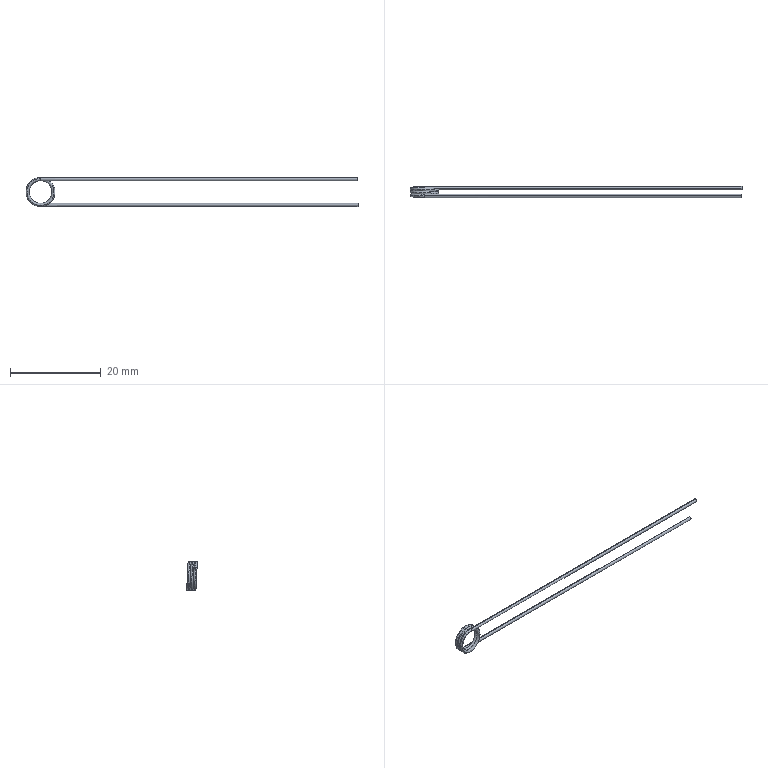Part | SolidWorks | features MoveFace 2, CompositeCurve 1, Helix 1, Sweep 1 | 1 solid | 9 faces | box 73.25 x 2.45 x 6.4 mm | volume 70.525 mm3 | cylinder 4 | spline 3 | plane 2 | commonest cylinder face diameters 0.7 x4
STEP:
#1=CARTESIAN_POINT('',(70.05,1.75,-3.2));
#2=VERTEX_POINT('',#1);
#3=CARTESIAN_POINT('',(70.05,1.75,-2.5));
#4=VERTEX_POINT('',#3);
#5=CARTESIAN_POINT('',(70.05,1.75,-2.85));
#6=DIRECTION('',(1.,0.,0.));
#7=DIRECTION('',(0.,0.00009155,-1.));
#8=AXIS2_PLACEMENT_3D('',#5,#6,#7);
#9=CIRCLE('',#8,0.35);
#10=EDGE_CURVE('',#2,#4,#9,.T.);
#11=ORIENTED_EDGE('',*,*,#10,.F.);
#12=CARTESIAN_POINT('',(-0.000000536,1.75,-3.2));
#13=VERTEX_POINT('',#12);
#14=CARTESIAN_POINT('',(12.85,1.75,-3.2));
#15=DIRECTION('',(-1.,0.,0.));
#16=VECTOR('',#15,1000.);
#17=LINE('',#14,#16);
#18=EDGE_CURVE('',#2,#13,#17,.T.);
#19=ORIENTED_EDGE('',*,*,#18,.T.);
#20=CARTESIAN_POINT('',(-0.006305,2.074,-2.979));
#21=VERTEX_POINT('',#20);
#22=CARTESIAN_POINT('',(0.,1.75,-2.85));
#23=DIRECTION('',(1.,0.,0.));
#24=DIRECTION('',(0.,0.00009155,-1.));
#25=AXIS2_PLACEMENT_3D('',#22,#23,#24);
#26=CIRCLE('',#25,0.35);
#27=EDGE_CURVE('',#13,#21,#26,.T.);
#28=ORIENTED_EDGE('',*,*,#27,.T.);
#29=CARTESIAN_POINT('',(0.,1.75,-2.5));
#30=VERTEX_POINT('',#29);
#31=CARTESIAN_POINT('',(0.,1.75,-2.85));
#32=DIRECTION('',(1.,0.,0.));
#33=DIRECTION('',(0.,0.00009155,-1.));
#34=AXIS2_PLACEMENT_3D('',#31,#32,#33);
#35=CIRCLE('',#34,0.35);
#36=EDGE_CURVE('',#21,#30,#35,.T.);
#37=ORIENTED_EDGE('',*,*,#36,.T.);
#38=CARTESIAN_POINT('',(12.85,1.75,-2.5));
#39=DIRECTION('',(-1.,0.,0.));
#40=VECTOR('',#39,1000.);
#41=LINE('',#38,#40);
#42=EDGE_CURVE('',#4,#30,#41,.T.);
#43=ORIENTED_EDGE('',*,*,#42,.F.);
#44=EDGE_LOOP('',(#11,#19,#28,#37,#43));
#45=FACE_OUTER_BOUND('',#44,.T.);
#46=CARTESIAN_POINT('',(12.85,1.75,-2.85));
#47=DIRECTION('',(-1.,0.,0.));
#48=DIRECTION('',(0.,0.,1.));
#49=AXIS2_PLACEMENT_3D('',#46,#47,#48);
#50=CYLINDRICAL_SURFACE('',#49,0.35);
#51=ADVANCED_FACE('',(#45),#50,.T.);
#52=CARTESIAN_POINT('',(0.006305,0.3239,2.979));
#53=VERTEX_POINT('',#52);
#54=CARTESIAN_POINT('',(0.,0.,3.2));
#55=VERTEX_POINT('',#54);
#56=CARTESIAN_POINT('',(0.006305,0.3239,2.979));
#57=CARTESIAN_POINT('',(0.01048,0.2681,3.104));
#58=CARTESIAN_POINT('',(0.005425,0.1388,3.2));
#59=CARTESIAN_POINT('',(0.,0.,3.2));
#60=B_SPLINE_CURVE_WITH_KNOTS('',3,(#56,#57,#58,#59),.UNSPECIFIED.,.F.,.F.,(4,4),(0.00002721,0.1895),.UNSPECIFIED.);
#61=EDGE_CURVE('',#53,#55,#60,.T.);
#62=ORIENTED_EDGE('',*,*,#61,.T.);
#63=CARTESIAN_POINT('',(70.05,0.,3.2));
#64=VERTEX_POINT('',#63);
#65=CARTESIAN_POINT('',(0.,0.,3.2));
#66=DIRECTION('',(1.,0.,0.));
#67=VECTOR('',#66,1000.);
#68=LINE('',#65,#67);
#69=EDGE_CURVE('',#55,#64,#68,.T.);
#70=ORIENTED_EDGE('',*,*,#69,.T.);
#71=CARTESIAN_POINT('',(70.05,0.,2.5));
#72=VERTEX_POINT('',#71);
#73=CARTESIAN_POINT('',(70.05,0.,2.85));
#74=DIRECTION('',(-1.,0.,0.));
#75=DIRECTION('',(0.,0.,1.));
#76=AXIS2_PLACEMENT_3D('',#73,#74,#75);
#77=CIRCLE('',#76,0.35);
#78=EDGE_CURVE('',#64,#72,#77,.T.);
#79=ORIENTED_EDGE('',*,*,#78,.T.);
#80=CARTESIAN_POINT('',(0.,0.,2.5));
#81=VERTEX_POINT('',#80);
#82=CARTESIAN_POINT('',(0.,0.,2.5));
#83=DIRECTION('',(1.,0.,0.));
#84=VECTOR('',#83,1000.);
#85=LINE('',#82,#84);
#86=EDGE_CURVE('',#81,#72,#85,.T.);
#87=ORIENTED_EDGE('',*,*,#86,.F.);
#88=CARTESIAN_POINT('',(0.,0.,2.85));
#89=DIRECTION('',(-1.,0.,0.));
#90=DIRECTION('',(0.,0.,1.));
#91=AXIS2_PLACEMENT_3D('',#88,#89,#90);
#92=CIRCLE('',#91,0.35);
#93=EDGE_CURVE('',#53,#81,#92,.T.);
#94=ORIENTED_EDGE('',*,*,#93,.F.);
#95=EDGE_LOOP('',(#62,#70,#79,#87,#94));
#96=FACE_OUTER_BOUND('',#95,.T.);
#97=CARTESIAN_POINT('',(0.,0.,2.85));
#98=DIRECTION('',(1.,0.,0.));
#99=DIRECTION('',(0.,0.,-1.));
#100=AXIS2_PLACEMENT_3D('',#97,#98,#99);
#101=CYLINDRICAL_SURFACE('',#100,0.35);
#102=ADVANCED_FACE('',(#96),#101,.T.);
#103=ORIENTED_EDGE('',*,*,#18,.F.);
#104=CARTESIAN_POINT('',(70.05,1.75,-2.85));
#105=DIRECTION('',(1.,0.,0.));
#106=DIRECTION('',(0.,0.00009155,-1.));
#107=AXIS2_PLACEMENT_3D('',#104,#105,#106);
#108=CIRCLE('',#107,0.35);
#109=EDGE_CURVE('',#4,#2,#108,.T.);
#110=ORIENTED_EDGE('',*,*,#109,.F.);
#111=ORIENTED_EDGE('',*,*,#42,.T.);
#112=CARTESIAN_POINT('',(0.006304,1.426,-2.979));
#113=VERTEX_POINT('',#112);
#114=CARTESIAN_POINT('',(0.,1.75,-2.85));
#115=DIRECTION('',(1.,0.,0.));
#116=DIRECTION('',(0.,0.00009155,-1.));
#117=AXIS2_PLACEMENT_3D('',#114,#115,#116);
#118=CIRCLE('',#117,0.35);
#119=EDGE_CURVE('',#30,#113,#118,.T.);
#120=ORIENTED_EDGE('',*,*,#119,.T.);
#121=CARTESIAN_POINT('',(0.,1.75,-2.85));
#122=DIRECTION('',(1.,0.,0.));
#123=DIRECTION('',(0.,0.00009155,-1.));
#124=AXIS2_PLACEMENT_3D('',#121,#122,#123);
#125=CIRCLE('',#124,0.35);
#126=EDGE_CURVE('',#113,#13,#125,.T.);
#127=ORIENTED_EDGE('',*,*,#126,.T.);
#128=EDGE_LOOP('',(#103,#110,#111,#120,#127));
#129=FACE_OUTER_BOUND('',#128,.T.);
#130=CARTESIAN_POINT('',(12.85,1.75,-2.85));
#131=DIRECTION('',(-1.,0.,0.));
#132=DIRECTION('',(0.,0.,1.));
#133=AXIS2_PLACEMENT_3D('',#130,#131,#132);
#134=CYLINDRICAL_SURFACE('',#133,0.35);
#135=ADVANCED_FACE('',(#129),#134,.T.);
#136=ORIENTED_EDGE('',*,*,#36,.F.);
#137=CARTESIAN_POINT('',(0.006305,0.3239,2.979));
#138=CARTESIAN_POINT('',(-0.7712,0.3519,2.981));
#139=CARTESIAN_POINT('',(-1.545,0.381,2.663));
#140=CARTESIAN_POINT('',(-2.649,0.4392,1.566));
#141=CARTESIAN_POINT('',(-2.975,0.4683,0.7939));
#142=CARTESIAN_POINT('',(-2.98,0.5195,-0.5733));
#143=CARTESIAN_POINT('',(-2.806,0.5413,-1.156));
#144=CARTESIAN_POINT('',(-2.162,0.585,-2.13));
#145=CARTESIAN_POINT('',(-1.69,0.6069,-2.521));
#146=CARTESIAN_POINT('',(-0.4324,0.658,-3.048));
#147=CARTESIAN_POINT('',(0.405,0.6871,-3.052));
#148=CARTESIAN_POINT('',(1.67,0.7383,-2.534));
#149=CARTESIAN_POINT('',(2.142,0.7601,-2.15));
#150=CARTESIAN_POINT('',(2.795,0.8037,-1.182));
#151=CARTESIAN_POINT('',(2.976,0.8257,-0.5972));
#152=CARTESIAN_POINT('',(2.981,0.8768,0.7668));
#153=CARTESIAN_POINT('',(2.665,0.9058,1.542));
#154=CARTESIAN_POINT('',(1.702,0.957,2.513));
#155=CARTESIAN_POINT('',(1.167,0.9788,2.801));
#156=CARTESIAN_POINT('',(0.02248,1.022,3.035));
#157=CARTESIAN_POINT('',(-0.587,1.044,2.978));
#158=CARTESIAN_POINT('',(-1.849,1.096,2.461));
#159=CARTESIAN_POINT('',(-2.445,1.125,1.872));
#160=CARTESIAN_POINT('',(-2.973,1.176,0.6109));
#161=CARTESIAN_POINT('',(-3.035,1.198,0.005944));
#162=CARTESIAN_POINT('',(-2.812,1.241,-1.14));
#163=CARTESIAN_POINT('',(-2.526,1.263,-1.682));
#164=CARTESIAN_POINT('',(-1.566,1.314,-2.65));
#165=CARTESIAN_POINT('',(-0.7938,1.343,-2.975));
#166=CARTESIAN_POINT('',(0.5733,1.395,-2.98));
#167=CARTESIAN_POINT('',(1.156,1.416,-2.806));
#168=CARTESIAN_POINT('',(2.13,1.46,-2.162));
#169=CARTESIAN_POINT('',(2.521,1.482,-1.69));
#170=CARTESIAN_POINT('',(3.048,1.533,-0.4324));
#171=CARTESIAN_POINT('',(3.052,1.562,0.405));
#172=CARTESIAN_POINT('',(2.534,1.613,1.67));
#173=CARTESIAN_POINT('',(2.15,1.635,2.142));
#174=CARTESIAN_POINT('',(1.182,1.679,2.795));
#175=CARTESIAN_POINT('',(0.5972,1.701,2.976));
#176=CARTESIAN_POINT('',(-0.7668,1.752,2.981));
#177=CARTESIAN_POINT('',(-1.542,1.781,2.665));
#178=CARTESIAN_POINT('',(-2.513,1.832,1.702));
#179=CARTESIAN_POINT('',(-2.801,1.854,1.167));
#180=CARTESIAN_POINT('',(-3.034,1.897,0.0225));
#181=CARTESIAN_POINT('',(-2.978,1.919,-0.587));
#182=CARTESIAN_POINT('',(-2.46,1.971,-1.85));
#183=CARTESIAN_POINT('',(-1.872,2.,-2.445));
#184=CARTESIAN_POINT('',(-0.7917,2.043,-2.897));
#185=CARTESIAN_POINT('',(-0.4042,2.058,-2.976));
#186=CARTESIAN_POINT('',(-0.006305,2.074,-2.979));
#187=B_SPLINE_CURVE_WITH_KNOTS('',3,(#137,#138,#139,#140,#141,#142,#143,#144,#145,#146,#147,#148,#149,#150,#151,#152,#153,#154,#155,#156,#157,#158,#159,#160,#161,#162,#163,#164,#165,#166,#167,#168,#169,#170,#171,#172,#173,#174,#175,#176,#177,#178,#179,#180,#181,#182,#183,#184,#185,#186),.UNSPECIFIED.,.F.,.F.,(4,2,2,2,2,2,2,2,2,2,2,2,2,2,2,2,2,2,2,2,2,2,2,2,4),(0.,0.04998,0.09999,0.1375,0.175,0.225,0.2625,0.3,0.35,0.3875,0.425,0.475,0.5125,0.55,0.6,0.6375,0.675,0.725,0.7625,0.8,0.85,0.8875,0.925,0.975,1.),.UNSPECIFIED.);
#188=EDGE_CURVE('',#53,#21,#187,.T.);
#189=ORIENTED_EDGE('',*,*,#188,.F.);
#190=ORIENTED_EDGE('',*,*,#93,.T.);
#191=CARTESIAN_POINT('',(-0.006304,-0.3239,2.979));
#192=VERTEX_POINT('',#191);
#193=CARTESIAN_POINT('',(0.,0.,2.85));
#194=DIRECTION('',(-1.,0.,0.));
#195=DIRECTION('',(0.,0.,1.));
#196=AXIS2_PLACEMENT_3D('',#193,#194,#195);
#197=CIRCLE('',#196,0.35);
#198=EDGE_CURVE('',#81,#192,#197,.T.);
#199=ORIENTED_EDGE('',*,*,#198,.T.);
#200=CARTESIAN_POINT('',(0.006304,1.426,-2.979));
#201=CARTESIAN_POINT('',(-0.379,1.413,-2.98));
#202=CARTESIAN_POINT('',(-0.7673,1.398,-2.904));
#203=CARTESIAN_POINT('',(-1.851,1.354,-2.461));
#204=CARTESIAN_POINT('',(-2.445,1.325,-1.871));
#205=CARTESIAN_POINT('',(-2.973,1.274,-0.6122));
#206=CARTESIAN_POINT('',(-3.035,1.252,-0.003211));
#207=CARTESIAN_POINT('',(-2.811,1.209,1.143));
#208=CARTESIAN_POINT('',(-2.527,1.187,1.681));
#209=CARTESIAN_POINT('',(-1.565,1.136,2.652));
#210=CARTESIAN_POINT('',(-0.792,1.107,2.975));
#211=CARTESIAN_POINT('',(0.572,1.056,2.981));
#212=CARTESIAN_POINT('',(1.158,1.034,2.805));
#213=CARTESIAN_POINT('',(2.132,0.99,2.16));
#214=CARTESIAN_POINT('',(2.52,0.9682,1.692));
#215=CARTESIAN_POINT('',(3.049,0.917,0.4308));
#216=CARTESIAN_POINT('',(3.052,0.8879,-0.4067));
#217=CARTESIAN_POINT('',(2.535,0.8368,-1.669));
#218=CARTESIAN_POINT('',(2.148,0.8149,-2.144));
#219=CARTESIAN_POINT('',(1.18,0.7712,-2.796));
#220=CARTESIAN_POINT('',(0.5985,0.7494,-2.976));
#221=CARTESIAN_POINT('',(-0.7686,0.6982,-2.981));
#222=CARTESIAN_POINT('',(-1.544,0.6692,-2.664));
#223=CARTESIAN_POINT('',(-2.512,0.6181,-1.703));
#224=CARTESIAN_POINT('',(-2.802,0.5961,-1.164));
#225=CARTESIAN_POINT('',(-3.035,0.5525,-0.01977));
#226=CARTESIAN_POINT('',(-2.978,0.5307,0.5858));
#227=CARTESIAN_POINT('',(-2.46,0.4795,1.851));
#228=CARTESIAN_POINT('',(-1.87,0.4504,2.445));
#229=CARTESIAN_POINT('',(-0.6122,0.3993,2.973));
#230=CARTESIAN_POINT('',(-0.003226,0.3774,3.035));
#231=CARTESIAN_POINT('',(1.143,0.3337,2.811));
#232=CARTESIAN_POINT('',(1.681,0.3119,2.527));
#233=CARTESIAN_POINT('',(2.652,0.2607,1.565));
#234=CARTESIAN_POINT('',(2.975,0.2317,0.792));
#235=CARTESIAN_POINT('',(2.981,0.1806,-0.572));
#236=CARTESIAN_POINT('',(2.805,0.1586,-1.158));
#237=CARTESIAN_POINT('',(2.16,0.115,-2.132));
#238=CARTESIAN_POINT('',(1.692,0.09317,-2.52));
#239=CARTESIAN_POINT('',(0.4308,0.04196,-3.049));
#240=CARTESIAN_POINT('',(-0.4067,0.01292,-3.052));
#241=CARTESIAN_POINT('',(-1.669,-0.03818,-2.535));
#242=CARTESIAN_POINT('',(-2.144,-0.06013,-2.148));
#243=CARTESIAN_POINT('',(-2.796,-0.1038,-1.18));
#244=CARTESIAN_POINT('',(-2.976,-0.1256,-0.5985));
#245=CARTESIAN_POINT('',(-2.981,-0.1768,0.7687));
#246=CARTESIAN_POINT('',(-2.663,-0.2059,1.544));
#247=CARTESIAN_POINT('',(-1.567,-0.2642,2.65));
#248=CARTESIAN_POINT('',(-0.7966,-0.2932,2.975));
#249=CARTESIAN_POINT('',(-0.006304,-0.3239,2.979));
#250=B_SPLINE_CURVE_WITH_KNOTS('',3,(#200,#201,#202,#203,#204,#205,#206,#207,#208,#209,#210,#211,#212,#213,#214,#215,#216,#217,#218,#219,#220,#221,#222,#223,#224,#225,#226,#227,#228,#229,#230,#231,#232,#233,#234,#235,#236,#237,#238,#239,#240,#241,#242,#243,#244,#245,#246,#247,#248,#249),.UNSPECIFIED.,.F.,.F.,(4,2,2,2,2,2,2,2,2,2,2,2,2,2,2,2,2,2,2,2,2,2,2,2,4),(0.,0.02496,0.07501,0.1125,0.15,0.2,0.2375,0.275,0.325,0.3625,0.4,0.45,0.4875,0.525,0.575,0.6125,0.65,0.7,0.7375,0.775,0.825,0.8625,0.9,0.95,1.),.UNSPECIFIED.);
#251=EDGE_CURVE('',#113,#192,#250,.T.);
#252=ORIENTED_EDGE('',*,*,#251,.F.);
#253=ORIENTED_EDGE('',*,*,#119,.F.);
#254=EDGE_LOOP('',(#136,#189,#190,#199,#252,#253));
#255=FACE_OUTER_BOUND('',#254,.T.);
#256=CARTESIAN_POINT('',(-0.01261,2.073,-2.978));
#257=CARTESIAN_POINT('',(-0.9931,2.036,-2.974));
#258=CARTESIAN_POINT('',(-1.942,2.,-2.452));
#259=CARTESIAN_POINT('',(-3.022,1.927,-0.8338));
#260=CARTESIAN_POINT('',(-3.123,1.89,0.2539));
#261=CARTESIAN_POINT('',(-2.369,1.817,2.048));
#262=CARTESIAN_POINT('',(-1.523,1.781,2.732));
#263=CARTESIAN_POINT('',(0.3864,1.708,3.111));
#264=CARTESIAN_POINT('',(1.43,1.671,2.788));
#265=CARTESIAN_POINT('',(2.798,1.599,1.405));
#266=CARTESIAN_POINT('',(3.107,1.562,0.3615));
#267=CARTESIAN_POINT('',(2.726,1.489,-1.547));
#268=CARTESIAN_POINT('',(2.029,1.453,-2.388));
#269=CARTESIAN_POINT('',(0.2273,1.38,-3.123));
#270=CARTESIAN_POINT('',(-0.8551,1.343,-3.009));
#271=CARTESIAN_POINT('',(-2.473,1.271,-1.927));
#272=CARTESIAN_POINT('',(-2.982,1.234,-0.9604));
#273=CARTESIAN_POINT('',(-2.972,1.161,0.9852));
#274=CARTESIAN_POINT('',(-2.453,1.125,1.942));
#275=CARTESIAN_POINT('',(-0.8335,1.052,3.022));
#276=CARTESIAN_POINT('',(0.2539,1.015,3.123));
#277=CARTESIAN_POINT('',(2.048,0.9425,2.369));
#278=CARTESIAN_POINT('',(2.732,0.9059,1.523));
#279=CARTESIAN_POINT('',(3.111,0.8331,-0.3864));
#280=CARTESIAN_POINT('',(2.788,0.7965,-1.43));
#281=CARTESIAN_POINT('',(1.405,0.7237,-2.798));
#282=CARTESIAN_POINT('',(0.3615,0.6872,-3.107));
#283=CARTESIAN_POINT('',(-1.547,0.6143,-2.726));
#284=CARTESIAN_POINT('',(-2.388,0.5777,-2.029));
#285=CARTESIAN_POINT('',(-3.123,0.505,-0.2273));
#286=CARTESIAN_POINT('',(-3.009,0.4684,0.8554));
#287=CARTESIAN_POINT('',(-1.927,0.3956,2.473));
#288=CARTESIAN_POINT('',(-0.9676,0.3593,2.982));
#289=CARTESIAN_POINT('',(0.01261,0.3226,2.978));
#290=CARTESIAN_POINT('',(-0.0161,2.162,-2.771));
#291=CARTESIAN_POINT('',(-0.9269,2.125,-2.766));
#292=CARTESIAN_POINT('',(-1.811,2.089,-2.279));
#293=CARTESIAN_POINT('',(-2.813,2.016,-0.7712));
#294=CARTESIAN_POINT('',(-2.906,1.979,0.2409));
#295=CARTESIAN_POINT('',(-2.201,1.907,1.909));
#296=CARTESIAN_POINT('',(-1.413,1.87,2.545));
#297=CARTESIAN_POINT('',(0.3644,1.797,2.894));
#298=CARTESIAN_POINT('',(1.334,1.761,2.592));
#299=CARTESIAN_POINT('',(2.606,1.688,1.303));
#300=CARTESIAN_POINT('',(2.892,1.651,0.3318));
#301=CARTESIAN_POINT('',(2.535,1.579,-1.444));
#302=CARTESIAN_POINT('',(1.884,1.542,-2.225));
#303=CARTESIAN_POINT('',(0.2064,1.469,-2.907));
#304=CARTESIAN_POINT('',(-0.8001,1.433,-2.799));
#305=CARTESIAN_POINT('',(-2.304,1.36,-1.789));
#306=CARTESIAN_POINT('',(-2.777,1.323,-0.8894));
#307=CARTESIAN_POINT('',(-2.764,1.25,0.9216));
#308=CARTESIAN_POINT('',(-2.279,1.214,1.81));
#309=CARTESIAN_POINT('',(-0.771,1.141,2.814));
#310=CARTESIAN_POINT('',(0.2409,1.104,2.906));
#311=CARTESIAN_POINT('',(1.909,1.032,2.201));
#312=CARTESIAN_POINT('',(2.545,0.9951,1.413));
#313=CARTESIAN_POINT('',(2.894,0.9223,-0.3644));
#314=CARTESIAN_POINT('',(2.592,0.8857,-1.334));
#315=CARTESIAN_POINT('',(1.303,0.8129,-2.606));
#316=CARTESIAN_POINT('',(0.3318,0.7764,-2.892));
#317=CARTESIAN_POINT('',(-1.444,0.7035,-2.535));
#318=CARTESIAN_POINT('',(-2.225,0.667,-1.884));
#319=CARTESIAN_POINT('',(-2.907,0.5942,-0.2064));
#320=CARTESIAN_POINT('',(-2.798,0.5576,0.8003));
#321=CARTESIAN_POINT('',(-1.789,0.4848,2.304));
#322=CARTESIAN_POINT('',(-0.8958,0.4485,2.776));
#323=CARTESIAN_POINT('',(0.0161,0.4118,2.771));
#324=CARTESIAN_POINT('',(-0.008888,1.977,-2.5));
#325=CARTESIAN_POINT('',(-0.8283,1.941,-2.497));
#326=CARTESIAN_POINT('',(-1.629,1.904,-2.059));
#327=CARTESIAN_POINT('',(-2.536,1.832,-0.7012));
#328=CARTESIAN_POINT('',(-2.622,1.795,0.2114));
#329=CARTESIAN_POINT('',(-1.989,1.722,1.718));
#330=CARTESIAN_POINT('',(-1.28,1.686,2.292));
#331=CARTESIAN_POINT('',(0.3232,1.613,2.612));
#332=CARTESIAN_POINT('',(1.199,1.576,2.341));
#333=CARTESIAN_POINT('',(2.349,1.503,1.18));
#334=CARTESIAN_POINT('',(2.608,1.467,0.3051));
#335=CARTESIAN_POINT('',(2.29,1.394,-1.298));
#336=CARTESIAN_POINT('',(1.704,1.358,-2.003));
#337=CARTESIAN_POINT('',(0.1914,1.285,-2.622));
#338=CARTESIAN_POINT('',(-0.716,1.248,-2.526));
#339=CARTESIAN_POINT('',(-2.075,1.175,-1.618));
#340=CARTESIAN_POINT('',(-2.503,1.139,-0.808));
#341=CARTESIAN_POINT('',(-2.495,1.066,0.8264));
#342=CARTESIAN_POINT('',(-2.06,1.029,1.628));
#343=CARTESIAN_POINT('',(-0.701,0.9565,2.537));
#344=CARTESIAN_POINT('',(0.2114,0.92,2.622));
#345=CARTESIAN_POINT('',(1.718,0.8471,1.989));
#346=CARTESIAN_POINT('',(2.292,0.8107,1.28));
#347=CARTESIAN_POINT('',(2.612,0.7378,-0.3232));
#348=CARTESIAN_POINT('',(2.341,0.7013,-1.199));
#349=CARTESIAN_POINT('',(1.18,0.6284,-2.349));
#350=CARTESIAN_POINT('',(0.3051,0.5919,-2.608));
#351=CARTESIAN_POINT('',(-1.298,0.519,-2.29));
#352=CARTESIAN_POINT('',(-2.003,0.4825,-1.704));
#353=CARTESIAN_POINT('',(-2.622,0.4096,-0.1914));
#354=CARTESIAN_POINT('',(-2.525,0.3732,0.7162));
#355=CARTESIAN_POINT('',(-1.619,0.3003,2.075));
#356=CARTESIAN_POINT('',(-0.8134,0.2639,2.503));
#357=CARTESIAN_POINT('',(0.008889,0.2274,2.5));
#358=CARTESIAN_POINT('',(0.008895,1.522,-2.5));
#359=CARTESIAN_POINT('',(-0.8105,1.486,-2.503));
#360=CARTESIAN_POINT('',(-1.614,1.45,-2.071));
#361=CARTESIAN_POINT('',(-2.532,1.377,-0.7193));
#362=CARTESIAN_POINT('',(-2.623,1.34,0.1927));
#363=CARTESIAN_POINT('',(-2.001,1.267,1.704));
#364=CARTESIAN_POINT('',(-1.296,1.231,2.283));
#365=CARTESIAN_POINT('',(0.3046,1.158,2.614));
#366=CARTESIAN_POINT('',(1.182,1.121,2.35));
#367=CARTESIAN_POINT('',(2.341,1.048,1.197));
#368=CARTESIAN_POINT('',(2.606,1.012,0.3236));
#369=CARTESIAN_POINT('',(2.299,0.9391,-1.282));
#370=CARTESIAN_POINT('',(1.719,0.9026,-1.991));
#371=CARTESIAN_POINT('',(0.2101,0.8297,-2.62));
#372=CARTESIAN_POINT('',(-0.6981,0.7933,-2.531));
#373=CARTESIAN_POINT('',(-2.064,0.7204,-1.633));
#374=CARTESIAN_POINT('',(-2.497,0.6839,-0.8259));
#375=CARTESIAN_POINT('',(-2.501,0.611,0.8087));
#376=CARTESIAN_POINT('',(-2.071,0.5745,1.614));
#377=CARTESIAN_POINT('',(-0.7191,0.5016,2.532));
#378=CARTESIAN_POINT('',(0.1927,0.4651,2.623));
#379=CARTESIAN_POINT('',(1.704,0.3922,2.001));
#380=CARTESIAN_POINT('',(2.283,0.3558,1.296));
#381=CARTESIAN_POINT('',(2.614,0.2829,-0.3046));
#382=CARTESIAN_POINT('',(2.35,0.2464,-1.182));
#383=CARTESIAN_POINT('',(1.197,0.1735,-2.341));
#384=CARTESIAN_POINT('',(0.3236,0.137,-2.606));
#385=CARTESIAN_POINT('',(-1.282,0.0641,-2.299));
#386=CARTESIAN_POINT('',(-1.991,0.02763,-1.719));
#387=CARTESIAN_POINT('',(-2.62,-0.04528,-0.2101));
#388=CARTESIAN_POINT('',(-2.531,-0.08173,0.6983));
#389=CARTESIAN_POINT('',(-1.633,-0.1546,2.064));
#390=CARTESIAN_POINT('',(-0.8313,-0.191,2.497));
#391=CARTESIAN_POINT('',(-0.008894,-0.2275,2.5));
#392=CARTESIAN_POINT('',(0.0161,1.338,-2.771));
#393=CARTESIAN_POINT('',(-0.8947,1.302,-2.777));
#394=CARTESIAN_POINT('',(-1.785,1.265,-2.3));
#395=CARTESIAN_POINT('',(-2.804,1.192,-0.804));
#396=CARTESIAN_POINT('',(-2.908,1.156,0.2071));
#397=CARTESIAN_POINT('',(-2.223,1.083,1.884));
#398=CARTESIAN_POINT('',(-1.443,1.046,2.528));
#399=CARTESIAN_POINT('',(0.3307,0.9736,2.899));
#400=CARTESIAN_POINT('',(1.304,0.937,2.608));
#401=CARTESIAN_POINT('',(2.591,0.8642,1.333));
#402=CARTESIAN_POINT('',(2.888,0.8277,0.3653));
#403=CARTESIAN_POINT('',(2.552,0.7548,-1.415));
#404=CARTESIAN_POINT('',(1.91,0.7183,-2.203));
#405=CARTESIAN_POINT('',(0.2402,0.6455,-2.904));
#406=CARTESIAN_POINT('',(-0.7677,0.6089,-2.808));
#407=CARTESIAN_POINT('',(-2.284,0.5361,-1.816));
#408=CARTESIAN_POINT('',(-2.766,0.4995,-0.9217));
#409=CARTESIAN_POINT('',(-2.775,0.4267,0.8895));
#410=CARTESIAN_POINT('',(-2.3,0.3902,1.784));
#411=CARTESIAN_POINT('',(-0.8038,0.3173,2.805));
#412=CARTESIAN_POINT('',(0.2071,0.2808,2.908));
#413=CARTESIAN_POINT('',(1.884,0.208,2.223));
#414=CARTESIAN_POINT('',(2.528,0.1714,1.443));
#415=CARTESIAN_POINT('',(2.899,0.09857,-0.3307));
#416=CARTESIAN_POINT('',(2.608,0.06204,-1.304));
#417=CARTESIAN_POINT('',(1.333,-0.01079,-2.591));
#418=CARTESIAN_POINT('',(0.3653,-0.0473,-2.888));
#419=CARTESIAN_POINT('',(-1.415,-0.1202,-2.552));
#420=CARTESIAN_POINT('',(-2.203,-0.1567,-1.91));
#421=CARTESIAN_POINT('',(-2.904,-0.2295,-0.2402));
#422=CARTESIAN_POINT('',(-2.807,-0.2661,0.7679));
#423=CARTESIAN_POINT('',(-1.816,-0.3389,2.283));
#424=CARTESIAN_POINT('',(-0.9282,-0.3752,2.766));
#425=CARTESIAN_POINT('',(-0.0161,-0.4119,2.771));
#426=CARTESIAN_POINT('',(0.01261,1.427,-2.978));
#427=CARTESIAN_POINT('',(-0.9679,1.391,-2.982));
#428=CARTESIAN_POINT('',(-1.922,1.354,-2.469));
#429=CARTESIAN_POINT('',(-3.015,1.282,-0.8595));
#430=CARTESIAN_POINT('',(-3.125,1.245,0.2275));
#431=CARTESIAN_POINT('',(-2.386,1.172,2.028));
#432=CARTESIAN_POINT('',(-1.546,1.136,2.72));
#433=CARTESIAN_POINT('',(0.36,1.063,3.114));
#434=CARTESIAN_POINT('',(1.406,1.026,2.8));
#435=CARTESIAN_POINT('',(2.787,0.9536,1.429));
#436=CARTESIAN_POINT('',(3.104,0.917,0.3878));
#437=CARTESIAN_POINT('',(2.739,0.8442,-1.524));
#438=CARTESIAN_POINT('',(2.049,0.8076,-2.37));
#439=CARTESIAN_POINT('',(0.2537,0.7349,-3.121));
#440=CARTESIAN_POINT('',(-0.8297,0.6983,-3.016));
#441=CARTESIAN_POINT('',(-2.457,0.6254,-1.948));
#442=CARTESIAN_POINT('',(-2.974,0.5889,-0.9857));
#443=CARTESIAN_POINT('',(-2.981,0.5161,0.96));
#444=CARTESIAN_POINT('',(-2.469,0.4795,1.921));
#445=CARTESIAN_POINT('',(-0.8592,0.4067,3.015));
#446=CARTESIAN_POINT('',(0.2275,0.3701,3.125));
#447=CARTESIAN_POINT('',(2.028,0.2974,2.386));
#448=CARTESIAN_POINT('',(2.72,0.2608,1.546));
#449=CARTESIAN_POINT('',(3.114,0.1879,-0.36));
#450=CARTESIAN_POINT('',(2.8,0.1514,-1.406));
#451=CARTESIAN_POINT('',(1.429,0.07861,-2.787));
#452=CARTESIAN_POINT('',(0.3878,0.04204,-3.104));
#453=CARTESIAN_POINT('',(-1.524,-0.03081,-2.739));
#454=CARTESIAN_POINT('',(-2.371,-0.06738,-2.049));
#455=CARTESIAN_POINT('',(-3.121,-0.1401,-0.2537));
#456=CARTESIAN_POINT('',(-3.016,-0.1767,0.83));
#457=CARTESIAN_POINT('',(-1.948,-0.2496,2.456));
#458=CARTESIAN_POINT('',(-0.993,-0.2858,2.974));
#459=CARTESIAN_POINT('',(-0.01261,-0.3225,2.978));
#460=B_SPLINE_SURFACE_WITH_KNOTS('',3,3,((#256,#257,#258,#259,#260,#261,#262,#263,#264,#265,#266,#267,#268,#269,#270,#271,#272,#273,#274,#275,#276,#277,#278,#279,#280,#281,#282,#283,#284,#285,#286,#287,#288,#289),(#290,#291,#292,#293,#294,#295,#296,#297,#298,#299,#300,#301,#302,#303,#304,#305,#306,#307,#308,#309,#310,#311,#312,#313,#314,#315,#316,#317,#318,#319,#320,#321,#322,#323),(#324,#325,#326,#327,#328,#329,#330,#331,#332,#333,#334,#335,#336,#337,#338,#339,#340,#341,#342,#343,#344,#345,#346,#347,#348,#349,#350,#351,#352,#353,#354,#355,#356,#357),(#358,#359,#360,#361,#362,#363,#364,#365,#366,#367,#368,#369,#370,#371,#372,#373,#374,#375,#376,#377,#378,#379,#380,#381,#382,#383,#384,#385,#386,#387,#388,#389,#390,#391),(#392,#393,#394,#395,#396,#397,#398,#399,#400,#401,#402,#403,#404,#405,#406,#407,#408,#409,#410,#411,#412,#413,#414,#415,#416,#417,#418,#419,#420,#421,#422,#423,#424,#425),(#426,#427,#428,#429,#430,#431,#432,#433,#434,#435,#436,#437,#438,#439,#440,#441,#442,#443,#444,#445,#446,#447,#448,#449,#450,#451,#452,#453,#454,#455,#456,#457,#458,#459)),.UNSPECIFIED.,.F.,.F.,.F.,(4,2,4),(4,2,2,2,2,2,2,2,2,2,2,2,2,2,2,2,4),(0.1895,0.5,0.8106),(0.,0.0625,0.125,0.1875,0.25,0.3125,0.375,0.4375,0.5,0.5625,0.625,0.6875,0.75,0.8125,0.875,0.9375,1.),.UNSPECIFIED.);
#461=ADVANCED_FACE('',(#255),#460,.F.);
#462=ORIENTED_EDGE('',*,*,#126,.F.);
#463=ORIENTED_EDGE('',*,*,#251,.T.);
#464=CARTESIAN_POINT('',(0.,0.,3.2));
#465=CARTESIAN_POINT('',(-0.005423,-0.1387,3.2));
#466=CARTESIAN_POINT('',(-0.01048,-0.268,3.104));
#467=CARTESIAN_POINT('',(-0.006304,-0.3239,2.979));
#468=B_SPLINE_CURVE_WITH_KNOTS('',3,(#464,#465,#466,#467),.UNSPECIFIED.,.F.,.F.,(4,4),(0.8106,1.),.UNSPECIFIED.);
#469=EDGE_CURVE('',#55,#192,#468,.T.);
#470=ORIENTED_EDGE('',*,*,#469,.F.);
#471=CARTESIAN_POINT('',(-0.000000536,1.75,-3.2));
#472=CARTESIAN_POINT('',(-0.4215,1.735,-3.2));
#473=CARTESIAN_POINT('',(-0.8371,1.721,-3.117));
#474=CARTESIAN_POINT('',(-2.001,1.677,-2.635));
#475=CARTESIAN_POINT('',(-2.635,1.648,-2.));
#476=CARTESIAN_POINT('',(-3.197,1.597,-0.6438));
#477=CARTESIAN_POINT('',(-3.261,1.575,0.01064));
#478=CARTESIAN_POINT('',(-3.015,1.531,1.241));
#479=CARTESIAN_POINT('',(-2.708,1.51,1.817));
#480=CARTESIAN_POINT('',(-1.669,1.458,2.857));
#481=CARTESIAN_POINT('',(-0.8382,1.429,3.2));
#482=CARTESIAN_POINT('',(0.6287,1.378,3.2));
#483=CARTESIAN_POINT('',(1.258,1.356,3.008));
#484=CARTESIAN_POINT('',(2.3,1.313,2.311));
#485=CARTESIAN_POINT('',(2.715,1.291,1.807));
#486=CARTESIAN_POINT('',(3.278,1.239,0.4484));
#487=CARTESIAN_POINT('',(3.277,1.211,-0.4502));
#488=CARTESIAN_POINT('',(2.716,1.159,-1.805));
#489=CARTESIAN_POINT('',(2.298,1.137,-2.313));
#490=CARTESIAN_POINT('',(1.255,1.094,-3.01));
#491=CARTESIAN_POINT('',(0.6301,1.072,-3.2));
#492=CARTESIAN_POINT('',(-0.8402,1.021,-3.2));
#493=CARTESIAN_POINT('',(-1.67,0.9918,-2.855));
#494=CARTESIAN_POINT('',(-2.707,0.9406,-1.818));
#495=CARTESIAN_POINT('',(-3.017,0.9186,-1.238));
#496=CARTESIAN_POINT('',(-3.261,0.875,-0.007701));
#497=CARTESIAN_POINT('',(-3.198,0.8533,0.6424));
#498=CARTESIAN_POINT('',(-2.635,0.8019,2.001));
#499=CARTESIAN_POINT('',(-1.999,0.773,2.636));
#500=CARTESIAN_POINT('',(-0.6438,0.7218,3.197));
#501=CARTESIAN_POINT('',(0.01062,0.6999,3.261));
#502=CARTESIAN_POINT('',(1.241,0.6563,3.015));
#503=CARTESIAN_POINT('',(1.817,0.6345,2.708));
#504=CARTESIAN_POINT('',(2.857,0.5832,1.669));
#505=CARTESIAN_POINT('',(3.2,0.5543,0.8382));
#506=CARTESIAN_POINT('',(3.2,0.5031,-0.6287));
#507=CARTESIAN_POINT('',(3.008,0.4811,-1.258));
#508=CARTESIAN_POINT('',(2.311,0.4375,-2.3));
#509=CARTESIAN_POINT('',(1.807,0.4158,-2.715));
#510=CARTESIAN_POINT('',(0.4484,0.3644,-3.278));
#511=CARTESIAN_POINT('',(-0.4502,0.3355,-3.277));
#512=CARTESIAN_POINT('',(-1.805,0.2843,-2.716));
#513=CARTESIAN_POINT('',(-2.313,0.2624,-2.298));
#514=CARTESIAN_POINT('',(-3.01,0.2188,-1.255));
#515=CARTESIAN_POINT('',(-3.2,0.197,-0.6301));
#516=CARTESIAN_POINT('',(-3.2,0.1457,0.8403));
#517=CARTESIAN_POINT('',(-2.854,0.1167,1.671));
#518=CARTESIAN_POINT('',(-1.671,0.05831,2.854));
#519=CARTESIAN_POINT('',(-0.8425,0.02943,3.2));
#520=CARTESIAN_POINT('',(0.,0.,3.2));
#521=B_SPLINE_CURVE_WITH_KNOTS('',3,(#471,#472,#473,#474,#475,#476,#477,#478,#479,#480,#481,#482,#483,#484,#485,#486,#487,#488,#489,#490,#491,#492,#493,#494,#495,#496,#497,#498,#499,#500,#501,#502,#503,#504,#505,#506,#507,#508,#509,#510,#511,#512,#513,#514,#515,#516,#517,#518,#519,#520),.UNSPECIFIED.,.F.,.F.,(4,2,2,2,2,2,2,2,2,2,2,2,2,2,2,2,2,2,2,2,2,2,2,2,4),(0.,0.02496,0.07501,0.1125,0.15,0.2,0.2375,0.275,0.325,0.3625,0.4,0.45,0.4875,0.525,0.575,0.6125,0.65,0.7,0.7375,0.775,0.825,0.8625,0.9,0.95,1.),.UNSPECIFIED.);
#522=EDGE_CURVE('',#13,#55,#521,.T.);
#523=ORIENTED_EDGE('',*,*,#522,.F.);
#524=EDGE_LOOP('',(#462,#463,#470,#523));
#525=FACE_OUTER_BOUND('',#524,.T.);
#526=CARTESIAN_POINT('',(0.01261,1.427,-2.978));
#527=CARTESIAN_POINT('',(-0.379,1.413,-2.98));
#528=CARTESIAN_POINT('',(-0.7673,1.398,-2.904));
#529=CARTESIAN_POINT('',(-1.851,1.354,-2.461));
#530=CARTESIAN_POINT('',(-2.445,1.325,-1.871));
#531=CARTESIAN_POINT('',(-2.973,1.274,-0.6122));
#532=CARTESIAN_POINT('',(-3.035,1.252,-0.003211));
#533=CARTESIAN_POINT('',(-2.811,1.209,1.143));
#534=CARTESIAN_POINT('',(-2.527,1.187,1.681));
#535=CARTESIAN_POINT('',(-1.565,1.136,2.652));
#536=CARTESIAN_POINT('',(-0.792,1.107,2.975));
#537=CARTESIAN_POINT('',(0.572,1.056,2.981));
#538=CARTESIAN_POINT('',(1.158,1.034,2.805));
#539=CARTESIAN_POINT('',(2.132,0.99,2.16));
#540=CARTESIAN_POINT('',(2.52,0.9682,1.692));
#541=CARTESIAN_POINT('',(3.049,0.917,0.4308));
#542=CARTESIAN_POINT('',(3.052,0.8879,-0.4067));
#543=CARTESIAN_POINT('',(2.535,0.8368,-1.669));
#544=CARTESIAN_POINT('',(2.148,0.8149,-2.144));
#545=CARTESIAN_POINT('',(1.18,0.7712,-2.796));
#546=CARTESIAN_POINT('',(0.5985,0.7494,-2.976));
#547=CARTESIAN_POINT('',(-0.7686,0.6982,-2.981));
#548=CARTESIAN_POINT('',(-1.544,0.6692,-2.664));
#549=CARTESIAN_POINT('',(-2.512,0.6181,-1.703));
#550=CARTESIAN_POINT('',(-2.802,0.5961,-1.164));
#551=CARTESIAN_POINT('',(-3.035,0.5525,-0.01977));
#552=CARTESIAN_POINT('',(-2.978,0.5307,0.5858));
#553=CARTESIAN_POINT('',(-2.46,0.4795,1.851));
#554=CARTESIAN_POINT('',(-1.87,0.4504,2.445));
#555=CARTESIAN_POINT('',(-0.6122,0.3993,2.973));
#556=CARTESIAN_POINT('',(-0.003226,0.3774,3.035));
#557=CARTESIAN_POINT('',(1.143,0.3337,2.811));
#558=CARTESIAN_POINT('',(1.681,0.3119,2.527));
#559=CARTESIAN_POINT('',(2.652,0.2607,1.565));
#560=CARTESIAN_POINT('',(2.975,0.2317,0.792));
#561=CARTESIAN_POINT('',(2.981,0.1806,-0.572));
#562=CARTESIAN_POINT('',(2.805,0.1586,-1.158));
#563=CARTESIAN_POINT('',(2.16,0.115,-2.132));
#564=CARTESIAN_POINT('',(1.692,0.09317,-2.52));
#565=CARTESIAN_POINT('',(0.4308,0.04196,-3.049));
#566=CARTESIAN_POINT('',(-0.4067,0.01292,-3.052));
#567=CARTESIAN_POINT('',(-1.669,-0.03818,-2.535));
#568=CARTESIAN_POINT('',(-2.144,-0.06013,-2.148));
#569=CARTESIAN_POINT('',(-2.796,-0.1038,-1.18));
#570=CARTESIAN_POINT('',(-2.976,-0.1256,-0.5985));
#571=CARTESIAN_POINT('',(-2.981,-0.1768,0.7687));
#572=CARTESIAN_POINT('',(-2.663,-0.2059,1.544));
#573=CARTESIAN_POINT('',(-1.567,-0.2642,2.65));
#574=CARTESIAN_POINT('',(-0.7966,-0.2932,2.975));
#575=CARTESIAN_POINT('',(-0.01261,-0.3225,2.978));
#576=CARTESIAN_POINT('',(0.01048,1.482,-3.104));
#577=CARTESIAN_POINT('',(-0.3981,1.467,-3.106));
#578=CARTESIAN_POINT('',(-0.802,1.453,-3.026));
#579=CARTESIAN_POINT('',(-1.932,1.409,-2.563));
#580=CARTESIAN_POINT('',(-2.55,1.38,-1.948));
#581=CARTESIAN_POINT('',(-3.099,1.329,-0.6352));
#582=CARTESIAN_POINT('',(-3.163,1.307,-0.0004747));
#583=CARTESIAN_POINT('',(-2.929,1.263,1.194));
#584=CARTESIAN_POINT('',(-2.633,1.241,1.754));
#585=CARTESIAN_POINT('',(-1.628,1.19,2.766));
#586=CARTESIAN_POINT('',(-0.8233,1.161,3.102));
#587=CARTESIAN_POINT('',(0.5992,1.11,3.106));
#588=CARTESIAN_POINT('',(1.21,1.088,2.923));
#589=CARTESIAN_POINT('',(2.224,1.044,2.249));
#590=CARTESIAN_POINT('',(2.628,1.023,1.761));
#591=CARTESIAN_POINT('',(3.178,0.9714,0.4459));
#592=CARTESIAN_POINT('',(3.181,0.9425,-0.4263));
#593=CARTESIAN_POINT('',(2.641,0.8913,-1.742));
#594=CARTESIAN_POINT('',(2.237,0.8694,-2.236));
#595=CARTESIAN_POINT('',(1.227,0.8257,-2.915));
#596=CARTESIAN_POINT('',(0.6215,0.804,-3.102));
#597=CARTESIAN_POINT('',(-0.8043,0.7527,-3.107));
#598=CARTESIAN_POINT('',(-1.611,0.7237,-2.775));
#599=CARTESIAN_POINT('',(-2.62,0.6725,-1.773));
#600=CARTESIAN_POINT('',(-2.922,0.6506,-1.211));
#601=CARTESIAN_POINT('',(-3.163,0.607,-0.01804));
#602=CARTESIAN_POINT('',(-3.104,0.5852,0.613));
#603=CARTESIAN_POINT('',(-2.563,0.5339,1.932));
#604=CARTESIAN_POINT('',(-1.948,0.505,2.55));
#605=CARTESIAN_POINT('',(-0.6352,0.4538,3.099));
#606=CARTESIAN_POINT('',(-0.0004918,0.4319,3.163));
#607=CARTESIAN_POINT('',(1.194,0.3882,2.929));
#608=CARTESIAN_POINT('',(1.754,0.3665,2.633));
#609=CARTESIAN_POINT('',(2.766,0.3152,1.628));
#610=CARTESIAN_POINT('',(3.102,0.2862,0.8233));
#611=CARTESIAN_POINT('',(3.106,0.235,-0.5992));
#612=CARTESIAN_POINT('',(2.923,0.2131,-1.21));
#613=CARTESIAN_POINT('',(2.249,0.1695,-2.224));
#614=CARTESIAN_POINT('',(1.761,0.1477,-2.628));
#615=CARTESIAN_POINT('',(0.4459,0.09641,-3.178));
#616=CARTESIAN_POINT('',(-0.4263,0.06746,-3.181));
#617=CARTESIAN_POINT('',(-1.742,0.01629,-2.641));
#618=CARTESIAN_POINT('',(-2.236,-0.005646,-2.237));
#619=CARTESIAN_POINT('',(-2.915,-0.04927,-1.227));
#620=CARTESIAN_POINT('',(-3.102,-0.07105,-0.6215));
#621=CARTESIAN_POINT('',(-3.107,-0.1223,0.8044));
#622=CARTESIAN_POINT('',(-2.774,-0.1514,1.612));
#623=CARTESIAN_POINT('',(-1.631,-0.2097,2.763));
#624=CARTESIAN_POINT('',(-0.8278,-0.2386,3.102));
#625=CARTESIAN_POINT('',(-0.01048,-0.268,3.104));
#626=CARTESIAN_POINT('',(0.005423,1.611,-3.2));
#627=CARTESIAN_POINT('',(-0.416,1.597,-3.201));
#628=CARTESIAN_POINT('',(-0.8318,1.582,-3.118));
#629=CARTESIAN_POINT('',(-1.996,1.538,-2.639));
#630=CARTESIAN_POINT('',(-2.632,1.509,-2.004));
#631=CARTESIAN_POINT('',(-3.196,1.458,-0.6492));
#632=CARTESIAN_POINT('',(-3.261,1.436,0.005106));
#633=CARTESIAN_POINT('',(-3.018,1.393,1.236));
#634=CARTESIAN_POINT('',(-2.711,1.371,1.813));
#635=CARTESIAN_POINT('',(-1.673,1.319,2.854));
#636=CARTESIAN_POINT('',(-0.8436,1.291,3.199));
#637=CARTESIAN_POINT('',(0.6232,1.239,3.201));
#638=CARTESIAN_POINT('',(1.253,1.217,3.011));
#639=CARTESIAN_POINT('',(2.296,1.174,2.315));
#640=CARTESIAN_POINT('',(2.712,1.152,1.811));
#641=CARTESIAN_POINT('',(3.277,1.101,0.4539));
#642=CARTESIAN_POINT('',(3.278,1.072,-0.4446));
#643=CARTESIAN_POINT('',(2.719,1.021,-1.801));
#644=CARTESIAN_POINT('',(2.302,0.9986,-2.309));
#645=CARTESIAN_POINT('',(1.26,0.955,-3.007));
#646=CARTESIAN_POINT('',(0.6356,0.9333,-3.199));
#647=CARTESIAN_POINT('',(-0.8348,0.8819,-3.201));
#648=CARTESIAN_POINT('',(-1.665,0.853,-2.858));
#649=CARTESIAN_POINT('',(-2.704,0.8018,-1.823));
#650=CARTESIAN_POINT('',(-3.014,0.7799,-1.243));
#651=CARTESIAN_POINT('',(-3.261,0.7363,-0.01323));
#652=CARTESIAN_POINT('',(-3.199,0.7145,0.637));
#653=CARTESIAN_POINT('',(-2.638,0.6632,1.996));
#654=CARTESIAN_POINT('',(-2.003,0.6343,2.632));
#655=CARTESIAN_POINT('',(-0.6492,0.583,3.196));
#656=CARTESIAN_POINT('',(0.005088,0.5611,3.261));
#657=CARTESIAN_POINT('',(1.236,0.5175,3.018));
#658=CARTESIAN_POINT('',(1.813,0.4958,2.711));
#659=CARTESIAN_POINT('',(2.854,0.4444,1.673));
#660=CARTESIAN_POINT('',(3.199,0.4155,0.8437));
#661=CARTESIAN_POINT('',(3.201,0.3643,-0.6232));
#662=CARTESIAN_POINT('',(3.011,0.3424,-1.253));
#663=CARTESIAN_POINT('',(2.315,0.2988,-2.296));
#664=CARTESIAN_POINT('',(1.811,0.277,-2.712));
#665=CARTESIAN_POINT('',(0.4539,0.2257,-3.277));
#666=CARTESIAN_POINT('',(-0.4446,0.1968,-3.278));
#667=CARTESIAN_POINT('',(-1.801,0.1455,-2.719));
#668=CARTESIAN_POINT('',(-2.309,0.1236,-2.302));
#669=CARTESIAN_POINT('',(-3.007,0.08004,-1.26));
#670=CARTESIAN_POINT('',(-3.199,0.05826,-0.6356));
#671=CARTESIAN_POINT('',(-3.201,0.006904,0.8348));
#672=CARTESIAN_POINT('',(-2.857,-0.02205,1.666));
#673=CARTESIAN_POINT('',(-1.676,-0.08045,2.852));
#674=CARTESIAN_POINT('',(-0.848,-0.1093,3.199));
#675=CARTESIAN_POINT('',(-0.005424,-0.1388,3.2));
#676=CARTESIAN_POINT('',(-0.000001252,1.75,-3.2));
#677=CARTESIAN_POINT('',(-0.4215,1.735,-3.2));
#678=CARTESIAN_POINT('',(-0.8371,1.721,-3.117));
#679=CARTESIAN_POINT('',(-2.001,1.677,-2.635));
#680=CARTESIAN_POINT('',(-2.635,1.648,-2.));
#681=CARTESIAN_POINT('',(-3.197,1.597,-0.6438));
#682=CARTESIAN_POINT('',(-3.261,1.575,0.01064));
#683=CARTESIAN_POINT('',(-3.015,1.531,1.241));
#684=CARTESIAN_POINT('',(-2.708,1.51,1.817));
#685=CARTESIAN_POINT('',(-1.669,1.458,2.857));
#686=CARTESIAN_POINT('',(-0.8382,1.429,3.2));
#687=CARTESIAN_POINT('',(0.6287,1.378,3.2));
#688=CARTESIAN_POINT('',(1.258,1.356,3.008));
#689=CARTESIAN_POINT('',(2.3,1.313,2.311));
#690=CARTESIAN_POINT('',(2.715,1.291,1.807));
#691=CARTESIAN_POINT('',(3.278,1.239,0.4484));
#692=CARTESIAN_POINT('',(3.277,1.211,-0.4502));
#693=CARTESIAN_POINT('',(2.716,1.159,-1.805));
#694=CARTESIAN_POINT('',(2.298,1.137,-2.313));
#695=CARTESIAN_POINT('',(1.255,1.094,-3.01));
#696=CARTESIAN_POINT('',(0.6301,1.072,-3.2));
#697=CARTESIAN_POINT('',(-0.8402,1.021,-3.2));
#698=CARTESIAN_POINT('',(-1.67,0.9918,-2.855));
#699=CARTESIAN_POINT('',(-2.707,0.9406,-1.818));
#700=CARTESIAN_POINT('',(-3.017,0.9186,-1.238));
#701=CARTESIAN_POINT('',(-3.261,0.875,-0.007701));
#702=CARTESIAN_POINT('',(-3.198,0.8533,0.6424));
#703=CARTESIAN_POINT('',(-2.635,0.8019,2.001));
#704=CARTESIAN_POINT('',(-1.999,0.773,2.636));
#705=CARTESIAN_POINT('',(-0.6438,0.7218,3.197));
#706=CARTESIAN_POINT('',(0.01062,0.6999,3.261));
#707=CARTESIAN_POINT('',(1.241,0.6563,3.015));
#708=CARTESIAN_POINT('',(1.817,0.6345,2.708));
#709=CARTESIAN_POINT('',(2.857,0.5832,1.669));
#710=CARTESIAN_POINT('',(3.2,0.5543,0.8382));
#711=CARTESIAN_POINT('',(3.2,0.5031,-0.6287));
#712=CARTESIAN_POINT('',(3.008,0.4811,-1.258));
#713=CARTESIAN_POINT('',(2.311,0.4375,-2.3));
#714=CARTESIAN_POINT('',(1.807,0.4158,-2.715));
#715=CARTESIAN_POINT('',(0.4484,0.3644,-3.278));
#716=CARTESIAN_POINT('',(-0.4502,0.3355,-3.277));
#717=CARTESIAN_POINT('',(-1.805,0.2843,-2.716));
#718=CARTESIAN_POINT('',(-2.313,0.2624,-2.298));
#719=CARTESIAN_POINT('',(-3.01,0.2188,-1.255));
#720=CARTESIAN_POINT('',(-3.2,0.197,-0.6301));
#721=CARTESIAN_POINT('',(-3.2,0.1457,0.8403));
#722=CARTESIAN_POINT('',(-2.854,0.1167,1.671));
#723=CARTESIAN_POINT('',(-1.671,0.05831,2.854));
#724=CARTESIAN_POINT('',(-0.8425,0.02943,3.2));
#725=CARTESIAN_POINT('',(0.,0.,3.2));
#726=B_SPLINE_SURFACE_WITH_KNOTS('',3,3,((#526,#527,#528,#529,#530,#531,#532,#533,#534,#535,#536,#537,#538,#539,#540,#541,#542,#543,#544,#545,#546,#547,#548,#549,#550,#551,#552,#553,#554,#555,#556,#557,#558,#559,#560,#561,#562,#563,#564,#565,#566,#567,#568,#569,#570,#571,#572,#573,#574,#575),(#576,#577,#578,#579,#580,#581,#582,#583,#584,#585,#586,#587,#588,#589,#590,#591,#592,#593,#594,#595,#596,#597,#598,#599,#600,#601,#602,#603,#604,#605,#606,#607,#608,#609,#610,#611,#612,#613,#614,#615,#616,#617,#618,#619,#620,#621,#622,#623,#624,#625),(#626,#627,#628,#629,#630,#631,#632,#633,#634,#635,#636,#637,#638,#639,#640,#641,#642,#643,#644,#645,#646,#647,#648,#649,#650,#651,#652,#653,#654,#655,#656,#657,#658,#659,#660,#661,#662,#663,#664,#665,#666,#667,#668,#669,#670,#671,#672,#673,#674,#675),(#676,#677,#678,#679,#680,#681,#682,#683,#684,#685,#686,#687,#688,#689,#690,#691,#692,#693,#694,#695,#696,#697,#698,#699,#700,#701,#702,#703,#704,#705,#706,#707,#708,#709,#710,#711,#712,#713,#714,#715,#716,#717,#718,#719,#720,#721,#722,#723,#724,#725)),.UNSPECIFIED.,.F.,.F.,.F.,(4,4),(4,2,2,2,2,2,2,2,2,2,2,2,2,2,2,2,2,2,2,2,2,2,2,2,4),(0.8106,1.),(0.,0.02496,0.07501,0.1125,0.15,0.2,0.2375,0.275,0.325,0.3625,0.4,0.45,0.4875,0.525,0.575,0.6125,0.65,0.7,0.7375,0.775,0.825,0.8625,0.9,0.95,1.),.UNSPECIFIED.);
#727=ADVANCED_FACE('',(#525),#726,.F.);
#728=ORIENTED_EDGE('',*,*,#27,.F.);
#729=ORIENTED_EDGE('',*,*,#522,.T.);
#730=ORIENTED_EDGE('',*,*,#61,.F.);
#731=ORIENTED_EDGE('',*,*,#188,.T.);
#732=EDGE_LOOP('',(#728,#729,#730,#731));
#733=FACE_OUTER_BOUND('',#732,.T.);
#734=CARTESIAN_POINT('',(-0.000001252,1.75,-3.2));
#735=CARTESIAN_POINT('',(-0.4215,1.735,-3.2));
#736=CARTESIAN_POINT('',(-0.8371,1.721,-3.117));
#737=CARTESIAN_POINT('',(-2.001,1.677,-2.635));
#738=CARTESIAN_POINT('',(-2.635,1.648,-2.));
#739=CARTESIAN_POINT('',(-3.197,1.597,-0.6438));
#740=CARTESIAN_POINT('',(-3.261,1.575,0.01064));
#741=CARTESIAN_POINT('',(-3.015,1.531,1.241));
#742=CARTESIAN_POINT('',(-2.708,1.51,1.817));
#743=CARTESIAN_POINT('',(-1.669,1.458,2.857));
#744=CARTESIAN_POINT('',(-0.8382,1.429,3.2));
#745=CARTESIAN_POINT('',(0.6287,1.378,3.2));
#746=CARTESIAN_POINT('',(1.258,1.356,3.008));
#747=CARTESIAN_POINT('',(2.3,1.313,2.311));
#748=CARTESIAN_POINT('',(2.715,1.291,1.807));
#749=CARTESIAN_POINT('',(3.278,1.239,0.4484));
#750=CARTESIAN_POINT('',(3.277,1.211,-0.4502));
#751=CARTESIAN_POINT('',(2.716,1.159,-1.805));
#752=CARTESIAN_POINT('',(2.298,1.137,-2.313));
#753=CARTESIAN_POINT('',(1.255,1.094,-3.01));
#754=CARTESIAN_POINT('',(0.6301,1.072,-3.2));
#755=CARTESIAN_POINT('',(-0.8402,1.021,-3.2));
#756=CARTESIAN_POINT('',(-1.67,0.9918,-2.855));
#757=CARTESIAN_POINT('',(-2.707,0.9406,-1.818));
#758=CARTESIAN_POINT('',(-3.017,0.9186,-1.238));
#759=CARTESIAN_POINT('',(-3.261,0.875,-0.007701));
#760=CARTESIAN_POINT('',(-3.198,0.8533,0.6424));
#761=CARTESIAN_POINT('',(-2.635,0.8019,2.001));
#762=CARTESIAN_POINT('',(-1.999,0.773,2.636));
#763=CARTESIAN_POINT('',(-0.6438,0.7218,3.197));
#764=CARTESIAN_POINT('',(0.01062,0.6999,3.261));
#765=CARTESIAN_POINT('',(1.241,0.6563,3.015));
#766=CARTESIAN_POINT('',(1.817,0.6345,2.708));
#767=CARTESIAN_POINT('',(2.857,0.5832,1.669));
#768=CARTESIAN_POINT('',(3.2,0.5543,0.8382));
#769=CARTESIAN_POINT('',(3.2,0.5031,-0.6287));
#770=CARTESIAN_POINT('',(3.008,0.4811,-1.258));
#771=CARTESIAN_POINT('',(2.311,0.4375,-2.3));
#772=CARTESIAN_POINT('',(1.807,0.4158,-2.715));
#773=CARTESIAN_POINT('',(0.4484,0.3644,-3.278));
#774=CARTESIAN_POINT('',(-0.4502,0.3355,-3.277));
#775=CARTESIAN_POINT('',(-1.805,0.2843,-2.716));
#776=CARTESIAN_POINT('',(-2.313,0.2624,-2.298));
#777=CARTESIAN_POINT('',(-3.01,0.2188,-1.255));
#778=CARTESIAN_POINT('',(-3.2,0.197,-0.6301));
#779=CARTESIAN_POINT('',(-3.2,0.1457,0.8403));
#780=CARTESIAN_POINT('',(-2.854,0.1167,1.671));
#781=CARTESIAN_POINT('',(-1.671,0.05831,2.854));
#782=CARTESIAN_POINT('',(-0.8425,0.02943,3.2));
#783=CARTESIAN_POINT('',(0.,0.,3.2));
#784=CARTESIAN_POINT('',(-0.005427,1.889,-3.2));
#785=CARTESIAN_POINT('',(-0.4269,1.874,-3.199));
#786=CARTESIAN_POINT('',(-0.8423,1.86,-3.115));
#787=CARTESIAN_POINT('',(-2.005,1.816,-2.632));
#788=CARTESIAN_POINT('',(-2.639,1.787,-1.995));
#789=CARTESIAN_POINT('',(-3.198,1.736,-0.6384));
#790=CARTESIAN_POINT('',(-3.261,1.714,0.01617));
#791=CARTESIAN_POINT('',(-3.013,1.67,1.246));
#792=CARTESIAN_POINT('',(-2.705,1.648,1.822));
#793=CARTESIAN_POINT('',(-1.664,1.597,2.86));
#794=CARTESIAN_POINT('',(-0.8328,1.568,3.201));
#795=CARTESIAN_POINT('',(0.6341,1.517,3.199));
#796=CARTESIAN_POINT('',(1.263,1.495,3.006));
#797=CARTESIAN_POINT('',(2.304,1.451,2.307));
#798=CARTESIAN_POINT('',(2.718,1.43,1.802));
#799=CARTESIAN_POINT('',(3.279,1.378,0.4428));
#800=CARTESIAN_POINT('',(3.276,1.349,-0.4557));
#801=CARTESIAN_POINT('',(2.713,1.298,-1.81));
#802=CARTESIAN_POINT('',(2.294,1.276,-2.317));
#803=CARTESIAN_POINT('',(1.25,1.233,-3.012));
#804=CARTESIAN_POINT('',(0.6247,1.211,-3.201));
#805=CARTESIAN_POINT('',(-0.8456,1.159,-3.199));
#806=CARTESIAN_POINT('',(-1.675,1.131,-2.853));
#807=CARTESIAN_POINT('',(-2.71,1.079,-1.814));
#808=CARTESIAN_POINT('',(-3.019,1.057,-1.233));
#809=CARTESIAN_POINT('',(-3.261,1.014,-0.002169));
#810=CARTESIAN_POINT('',(-3.196,0.9921,0.6478));
#811=CARTESIAN_POINT('',(-2.632,0.9407,2.005));
#812=CARTESIAN_POINT('',(-1.995,0.9119,2.639));
#813=CARTESIAN_POINT('',(-0.6384,0.8606,3.198));
#814=CARTESIAN_POINT('',(0.01615,0.8387,3.261));
#815=CARTESIAN_POINT('',(1.246,0.7951,3.013));
#816=CARTESIAN_POINT('',(1.822,0.7733,2.705));
#817=CARTESIAN_POINT('',(2.86,0.722,1.664));
#818=CARTESIAN_POINT('',(3.201,0.6931,0.8328));
#819=CARTESIAN_POINT('',(3.199,0.6419,-0.6341));
#820=CARTESIAN_POINT('',(3.006,0.6199,-1.263));
#821=CARTESIAN_POINT('',(2.307,0.5763,-2.304));
#822=CARTESIAN_POINT('',(1.802,0.5546,-2.718));
#823=CARTESIAN_POINT('',(0.4428,0.5032,-3.279));
#824=CARTESIAN_POINT('',(-0.4557,0.4744,-3.276));
#825=CARTESIAN_POINT('',(-1.81,0.4231,-2.713));
#826=CARTESIAN_POINT('',(-2.317,0.4012,-2.294));
#827=CARTESIAN_POINT('',(-3.012,0.3576,-1.25));
#828=CARTESIAN_POINT('',(-3.201,0.3358,-0.6247));
#829=CARTESIAN_POINT('',(-3.199,0.2845,0.8457));
#830=CARTESIAN_POINT('',(-2.852,0.2555,1.675));
#831=CARTESIAN_POINT('',(-1.667,0.1971,2.857));
#832=CARTESIAN_POINT('',(-0.8371,0.1682,3.201));
#833=CARTESIAN_POINT('',(0.005426,0.1388,3.2));
#834=CARTESIAN_POINT('',(-0.01048,2.018,-3.104));
#835=CARTESIAN_POINT('',(-0.4191,2.003,-3.103));
#836=CARTESIAN_POINT('',(-0.8224,1.989,-3.02));
#837=CARTESIAN_POINT('',(-1.949,1.945,-2.55));
#838=CARTESIAN_POINT('',(-2.563,1.916,-1.931));
#839=CARTESIAN_POINT('',(-3.103,1.865,-0.6143));
#840=CARTESIAN_POINT('',(-3.163,1.843,0.02089));
#841=CARTESIAN_POINT('',(-2.921,1.799,1.214));
#842=CARTESIAN_POINT('',(-2.621,1.778,1.772));
#843=CARTESIAN_POINT('',(-1.61,1.726,2.777));
#844=CARTESIAN_POINT('',(-0.8024,1.697,3.107));
#845=CARTESIAN_POINT('',(0.6201,1.646,3.102));
#846=CARTESIAN_POINT('',(1.23,1.624,2.914));
#847=CARTESIAN_POINT('',(2.239,1.581,2.234));
#848=CARTESIAN_POINT('',(2.64,1.559,1.744));
#849=CARTESIAN_POINT('',(3.181,1.508,0.4245));
#850=CARTESIAN_POINT('',(3.177,1.479,-0.4477));
#851=CARTESIAN_POINT('',(2.629,1.427,-1.76));
#852=CARTESIAN_POINT('',(2.222,1.406,-2.251));
#853=CARTESIAN_POINT('',(1.207,1.362,-2.924));
#854=CARTESIAN_POINT('',(0.6006,1.34,-3.106));
#855=CARTESIAN_POINT('',(-0.8252,1.289,-3.102));
#856=CARTESIAN_POINT('',(-1.63,1.26,-2.764));
#857=CARTESIAN_POINT('',(-2.632,1.209,-1.755));
#858=CARTESIAN_POINT('',(-2.93,1.187,-1.191));
#859=CARTESIAN_POINT('',(-3.163,1.143,0.003325));
#860=CARTESIAN_POINT('',(-3.1,1.121,0.6338));
#861=CARTESIAN_POINT('',(-2.55,1.07,1.949));
#862=CARTESIAN_POINT('',(-1.93,1.041,2.563));
#863=CARTESIAN_POINT('',(-0.6143,0.9899,3.103));
#864=CARTESIAN_POINT('',(0.02088,0.968,3.163));
#865=CARTESIAN_POINT('',(1.214,0.9244,2.921));
#866=CARTESIAN_POINT('',(1.772,0.9026,2.621));
#867=CARTESIAN_POINT('',(2.777,0.8513,1.61));
#868=CARTESIAN_POINT('',(3.107,0.8224,0.8024));
#869=CARTESIAN_POINT('',(3.102,0.7712,-0.6201));
#870=CARTESIAN_POINT('',(2.914,0.7493,-1.23));
#871=CARTESIAN_POINT('',(2.234,0.7056,-2.239));
#872=CARTESIAN_POINT('',(1.744,0.6839,-2.64));
#873=CARTESIAN_POINT('',(0.4245,0.6326,-3.181));
#874=CARTESIAN_POINT('',(-0.4477,0.6036,-3.177));
#875=CARTESIAN_POINT('',(-1.76,0.5524,-2.629));
#876=CARTESIAN_POINT('',(-2.251,0.5305,-2.222));
#877=CARTESIAN_POINT('',(-2.924,0.4869,-1.207));
#878=CARTESIAN_POINT('',(-3.106,0.4651,-0.6006));
#879=CARTESIAN_POINT('',(-3.102,0.4138,0.8253));
#880=CARTESIAN_POINT('',(-2.763,0.3848,1.63));
#881=CARTESIAN_POINT('',(-1.612,0.3265,2.774));
#882=CARTESIAN_POINT('',(-0.8067,0.2975,3.107));
#883=CARTESIAN_POINT('',(0.01048,0.2681,3.104));
#884=CARTESIAN_POINT('',(-0.01261,2.073,-2.978));
#885=CARTESIAN_POINT('',(-0.4042,2.058,-2.976));
#886=CARTESIAN_POINT('',(-0.7917,2.043,-2.897));
#887=CARTESIAN_POINT('',(-1.872,2.,-2.445));
#888=CARTESIAN_POINT('',(-2.46,1.971,-1.85));
#889=CARTESIAN_POINT('',(-2.978,1.919,-0.587));
#890=CARTESIAN_POINT('',(-3.034,1.897,0.0225));
#891=CARTESIAN_POINT('',(-2.801,1.854,1.167));
#892=CARTESIAN_POINT('',(-2.513,1.832,1.702));
#893=CARTESIAN_POINT('',(-1.542,1.781,2.665));
#894=CARTESIAN_POINT('',(-0.7668,1.752,2.981));
#895=CARTESIAN_POINT('',(0.5972,1.701,2.976));
#896=CARTESIAN_POINT('',(1.182,1.679,2.795));
#897=CARTESIAN_POINT('',(2.15,1.635,2.142));
#898=CARTESIAN_POINT('',(2.534,1.613,1.67));
#899=CARTESIAN_POINT('',(3.052,1.562,0.405));
#900=CARTESIAN_POINT('',(3.048,1.533,-0.4324));
#901=CARTESIAN_POINT('',(2.521,1.482,-1.69));
#902=CARTESIAN_POINT('',(2.13,1.46,-2.162));
#903=CARTESIAN_POINT('',(1.156,1.416,-2.806));
#904=CARTESIAN_POINT('',(0.5733,1.395,-2.98));
#905=CARTESIAN_POINT('',(-0.7938,1.343,-2.975));
#906=CARTESIAN_POINT('',(-1.566,1.314,-2.65));
#907=CARTESIAN_POINT('',(-2.526,1.263,-1.682));
#908=CARTESIAN_POINT('',(-2.812,1.241,-1.14));
#909=CARTESIAN_POINT('',(-3.035,1.198,0.005944));
#910=CARTESIAN_POINT('',(-2.973,1.176,0.6109));
#911=CARTESIAN_POINT('',(-2.445,1.125,1.872));
#912=CARTESIAN_POINT('',(-1.849,1.096,2.461));
#913=CARTESIAN_POINT('',(-0.587,1.044,2.978));
#914=CARTESIAN_POINT('',(0.02248,1.022,3.035));
#915=CARTESIAN_POINT('',(1.167,0.9788,2.801));
#916=CARTESIAN_POINT('',(1.702,0.957,2.513));
#917=CARTESIAN_POINT('',(2.665,0.9058,1.542));
#918=CARTESIAN_POINT('',(2.981,0.8768,0.7668));
#919=CARTESIAN_POINT('',(2.976,0.8257,-0.5972));
#920=CARTESIAN_POINT('',(2.795,0.8037,-1.182));
#921=CARTESIAN_POINT('',(2.142,0.7601,-2.15));
#922=CARTESIAN_POINT('',(1.67,0.7383,-2.534));
#923=CARTESIAN_POINT('',(0.405,0.6871,-3.052));
#924=CARTESIAN_POINT('',(-0.4324,0.658,-3.048));
#925=CARTESIAN_POINT('',(-1.69,0.6069,-2.521));
#926=CARTESIAN_POINT('',(-2.162,0.585,-2.13));
#927=CARTESIAN_POINT('',(-2.806,0.5413,-1.156));
#928=CARTESIAN_POINT('',(-2.98,0.5195,-0.5733));
#929=CARTESIAN_POINT('',(-2.975,0.4683,0.7939));
#930=CARTESIAN_POINT('',(-2.649,0.4392,1.566));
#931=CARTESIAN_POINT('',(-1.545,0.381,2.663));
#932=CARTESIAN_POINT('',(-0.7712,0.3519,2.981));
#933=CARTESIAN_POINT('',(0.01261,0.3226,2.978));
#934=B_SPLINE_SURFACE_WITH_KNOTS('',3,3,((#734,#735,#736,#737,#738,#739,#740,#741,#742,#743,#744,#745,#746,#747,#748,#749,#750,#751,#752,#753,#754,#755,#756,#757,#758,#759,#760,#761,#762,#763,#764,#765,#766,#767,#768,#769,#770,#771,#772,#773,#774,#775,#776,#777,#778,#779,#780,#781,#782,#783),(#784,#785,#786,#787,#788,#789,#790,#791,#792,#793,#794,#795,#796,#797,#798,#799,#800,#801,#802,#803,#804,#805,#806,#807,#808,#809,#810,#811,#812,#813,#814,#815,#816,#817,#818,#819,#820,#821,#822,#823,#824,#825,#826,#827,#828,#829,#830,#831,#832,#833),(#834,#835,#836,#837,#838,#839,#840,#841,#842,#843,#844,#845,#846,#847,#848,#849,#850,#851,#852,#853,#854,#855,#856,#857,#858,#859,#860,#861,#862,#863,#864,#865,#866,#867,#868,#869,#870,#871,#872,#873,#874,#875,#876,#877,#878,#879,#880,#881,#882,#883),(#884,#885,#886,#887,#888,#889,#890,#891,#892,#893,#894,#895,#896,#897,#898,#899,#900,#901,#902,#903,#904,#905,#906,#907,#908,#909,#910,#911,#912,#913,#914,#915,#916,#917,#918,#919,#920,#921,#922,#923,#924,#925,#926,#927,#928,#929,#930,#931,#932,#933)),.UNSPECIFIED.,.F.,.F.,.F.,(4,4),(4,2,2,2,2,2,2,2,2,2,2,2,2,2,2,2,2,2,2,2,2,2,2,2,4),(0.,0.1895),(0.,0.02496,0.07501,0.1125,0.15,0.2,0.2375,0.275,0.325,0.3625,0.4,0.45,0.4875,0.525,0.575,0.6125,0.65,0.7,0.7375,0.775,0.825,0.8625,0.9,0.95,1.),.UNSPECIFIED.);
#935=ADVANCED_FACE('',(#733),#934,.F.);
#936=ORIENTED_EDGE('',*,*,#69,.F.);
#937=ORIENTED_EDGE('',*,*,#469,.T.);
#938=ORIENTED_EDGE('',*,*,#198,.F.);
#939=ORIENTED_EDGE('',*,*,#86,.T.);
#940=CARTESIAN_POINT('',(70.05,0.,2.85));
#941=DIRECTION('',(-1.,0.,0.));
#942=DIRECTION('',(0.,0.,1.));
#943=AXIS2_PLACEMENT_3D('',#940,#941,#942);
#944=CIRCLE('',#943,0.35);
#945=EDGE_CURVE('',#72,#64,#944,.T.);
#946=ORIENTED_EDGE('',*,*,#945,.T.);
#947=EDGE_LOOP('',(#936,#937,#938,#939,#946));
#948=FACE_OUTER_BOUND('',#947,.T.);
#949=CARTESIAN_POINT('',(0.,0.,2.85));
#950=DIRECTION('',(1.,0.,0.));
#951=DIRECTION('',(0.,0.,-1.));
#952=AXIS2_PLACEMENT_3D('',#949,#950,#951);
#953=CYLINDRICAL_SURFACE('',#952,0.35);
#954=ADVANCED_FACE('',(#948),#953,.T.);
#955=ORIENTED_EDGE('',*,*,#109,.T.);
#956=ORIENTED_EDGE('',*,*,#10,.T.);
#957=EDGE_LOOP('',(#955,#956));
#958=FACE_OUTER_BOUND('',#957,.T.);
#959=CARTESIAN_POINT('',(70.05,1.75,-2.85));
#960=DIRECTION('',(1.,0.,0.));
#961=DIRECTION('',(0.,0.00009155,-1.));
#962=AXIS2_PLACEMENT_3D('',#959,#960,#961);
#963=PLANE('',#962);
#964=ADVANCED_FACE('',(#958),#963,.T.);
#965=ORIENTED_EDGE('',*,*,#945,.F.);
#966=ORIENTED_EDGE('',*,*,#78,.F.);
#967=EDGE_LOOP('',(#965,#966));
#968=FACE_OUTER_BOUND('',#967,.T.);
#969=CARTESIAN_POINT('',(70.05,0.,2.85));
#970=DIRECTION('',(-1.,0.,0.));
#971=DIRECTION('',(0.,0.,1.));
#972=AXIS2_PLACEMENT_3D('',#969,#970,#971);
#973=PLANE('',#972);
#974=ADVANCED_FACE('',(#968),#973,.F.);
#975=CLOSED_SHELL('',(#51,#102,#135,#461,#727,#935,#954,#964,#974));
#976=MANIFOLD_SOLID_BREP('',#975);
#977=CARTESIAN_POINT('',(0.,0.,0.));
#978=DIRECTION('',(0.,0.,1.));
#979=DIRECTION('',(1.,0.,0.));
#980=AXIS2_PLACEMENT_3D('',#977,#978,#979);
#981=(LENGTH_UNIT()NAMED_UNIT(*)SI_UNIT(.MILLI.,.METRE.));
#982=UNCERTAINTY_MEASURE_WITH_UNIT(LENGTH_MEASURE(0.00001),#981,'','');
#983=(NAMED_UNIT(*)PLANE_ANGLE_UNIT()SI_UNIT($,.RADIAN.));
#984=(NAMED_UNIT(*)SI_UNIT($,.STERADIAN.)SOLID_ANGLE_UNIT());
#985=(GEOMETRIC_REPRESENTATION_CONTEXT(3)GLOBAL_UNCERTAINTY_ASSIGNED_CONTEXT((#982))GLOBAL_UNIT_ASSIGNED_CONTEXT((#981,#983,#984))REPRESENTATION_CONTEXT('',''));
#986=ADVANCED_BREP_SHAPE_REPRESENTATION('',(#976,#980),#985);